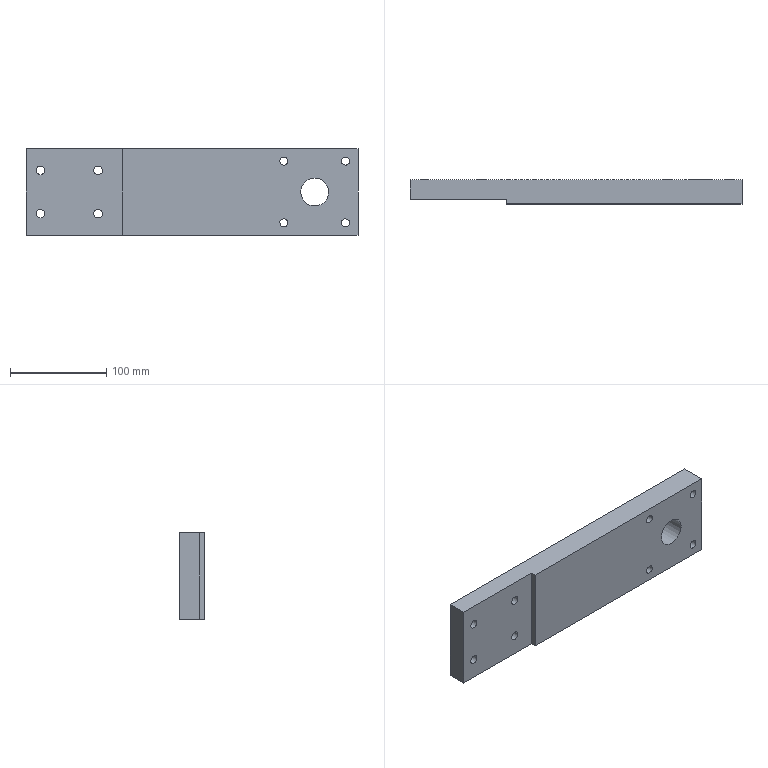Part | STEP file | SN10_001_007_PLACA | 1 solid | 17 faces | box 345 x 25 x 90 mm | volume 704137 mm3 | cylinder 9 | plane 8 | commonest cylinder face diameters 8.376 x4 9 x4 29 x1
STEP:
#1=CARTESIAN_POINT('',(0.,0.,0.));
#2=DIRECTION('',(0.,0.,1.));
#3=DIRECTION('',(1.,0.,0.));
#4=AXIS2_PLACEMENT_3D('',#1,#2,#3);
#5=CARTESIAN_POINT('',(5718.949,200.,-20.343));
#6=VERTEX_POINT('',#5);
#7=CARTESIAN_POINT('',(5715.,200.,-22.5));
#8=DIRECTION('',(0.,-1.,0.));
#9=DIRECTION('',(1.,0.,0.));
#10=AXIS2_PLACEMENT_3D('',#7,#8,#9);
#11=CIRCLE('',#10,4.5);
#12=CARTESIAN_POINT('',(5715.,199.9,-22.5));
#13=DIRECTION('',(0.,-1.,0.));
#14=DIRECTION('',(0.8776,0.,0.4794));
#15=AXIS2_PLACEMENT_3D('',#12,#13,#14);
#16=CYLINDRICAL_SURFACE('',#15,4.5);
#17=CARTESIAN_POINT('',(-0.5,-0.1));
#18=DIRECTION('',(1.,0.));
#19=VECTOR('',#18,1.);
#20=LINE('',#17,#19);
#21=(GEOMETRIC_REPRESENTATION_CONTEXT(2)PARAMETRIC_REPRESENTATION_CONTEXT()REPRESENTATION_CONTEXT('',''));
#22=DEFINITIONAL_REPRESENTATION('',(#20),#21);
#23=PCURVE('',#16,#22);
#24=CARTESIAN_POINT('',(6045.,200.,0.));
#25=DIRECTION('',(0.,1.,0.));
#26=DIRECTION('',(0.,0.,1.));
#27=AXIS2_PLACEMENT_3D('',#24,#25,#26);
#28=PLANE('',#27);
#29=CARTESIAN_POINT('',(-22.5,-325.5));
#30=CARTESIAN_POINT('',(-14.706,-325.5));
#31=CARTESIAN_POINT('',(-18.603,-332.25));
#32=CARTESIAN_POINT('',(-22.5,-339.));
#33=CARTESIAN_POINT('',(-26.397,-332.25));
#34=CARTESIAN_POINT('',(-30.294,-325.5));
#35=CARTESIAN_POINT('',(-22.5,-325.5));
#36=(BOUNDED_CURVE()B_SPLINE_CURVE(2,(#29,#30,#31,#32,#33,#34,#35),.UNSPECIFIED.,.T.,.F.)B_SPLINE_CURVE_WITH_KNOTS((1,2,2,2,2,1),(-2.094,0.,2.094,4.189,6.283,8.378),.UNSPECIFIED.)CURVE()GEOMETRIC_REPRESENTATION_ITEM()RATIONAL_B_SPLINE_CURVE((1.,0.5,1.,0.5,1.,0.5,1.))REPRESENTATION_ITEM(''));
#37=(GEOMETRIC_REPRESENTATION_CONTEXT(2)PARAMETRIC_REPRESENTATION_CONTEXT()REPRESENTATION_CONTEXT('',''));
#38=DEFINITIONAL_REPRESENTATION('',(#36),#37);
#39=PCURVE('',#28,#38);
#40=SURFACE_CURVE('',#11,(#23,#39),.PCURVE_S1.);
#41=EDGE_CURVE('',#6,#6,#40,.T.);
#42=ORIENTED_EDGE('',*,*,#41,.T.);
#43=CARTESIAN_POINT('',(5718.949,180.,-20.343));
#44=VERTEX_POINT('',#43);
#45=CARTESIAN_POINT('',(5718.949,200.,-20.343));
#46=CARTESIAN_POINT('',(5718.949,180.,-20.343));
#47=B_SPLINE_CURVE_WITH_KNOTS('',1,(#45,#46),.UNSPECIFIED.,.F.,.F.,(2,2),(-0.1,19.9),.PIECEWISE_BEZIER_KNOTS.);
#48=CARTESIAN_POINT('',(6.283,0.));
#49=DIRECTION('',(0.,1.));
#50=VECTOR('',#49,1.);
#51=LINE('',#48,#50);
#52=(GEOMETRIC_REPRESENTATION_CONTEXT(2)PARAMETRIC_REPRESENTATION_CONTEXT()REPRESENTATION_CONTEXT('',''));
#53=DEFINITIONAL_REPRESENTATION('',(#51),#52);
#54=PCURVE('',#16,#53);
#55=CARTESIAN_POINT('',(0.,0.));
#56=DIRECTION('',(0.,1.));
#57=VECTOR('',#56,1.);
#58=LINE('',#55,#57);
#59=(GEOMETRIC_REPRESENTATION_CONTEXT(2)PARAMETRIC_REPRESENTATION_CONTEXT()REPRESENTATION_CONTEXT('',''));
#60=DEFINITIONAL_REPRESENTATION('',(#58),#59);
#61=PCURVE('',#16,#60);
#62=SEAM_CURVE('',#47,(#54,#61),.PCURVE_S1.);
#63=EDGE_CURVE('',#6,#44,#62,.T.);
#64=ORIENTED_EDGE('',*,*,#63,.T.);
#65=CARTESIAN_POINT('',(5715.,180.,-22.5));
#66=DIRECTION('',(0.,-1.,0.));
#67=DIRECTION('',(1.,0.,0.));
#68=AXIS2_PLACEMENT_3D('',#65,#66,#67);
#69=CIRCLE('',#68,4.5);
#70=CARTESIAN_POINT('',(-0.5,19.9));
#71=DIRECTION('',(1.,0.));
#72=VECTOR('',#71,1.);
#73=LINE('',#70,#72);
#74=(GEOMETRIC_REPRESENTATION_CONTEXT(2)PARAMETRIC_REPRESENTATION_CONTEXT()REPRESENTATION_CONTEXT('',''));
#75=DEFINITIONAL_REPRESENTATION('',(#73),#74);
#76=PCURVE('',#16,#75);
#77=CARTESIAN_POINT('',(5700.,180.,0.));
#78=DIRECTION('',(0.,-1.,0.));
#79=DIRECTION('',(0.,0.,-1.));
#80=AXIS2_PLACEMENT_3D('',#77,#78,#79);
#81=PLANE('',#80);
#82=CARTESIAN_POINT('',(22.5,15.));
#83=DIRECTION('',(0.,1.));
#84=AXIS2_PLACEMENT_2D('',#82,#83);
#85=CIRCLE('',#84,4.5);
#86=(GEOMETRIC_REPRESENTATION_CONTEXT(2)PARAMETRIC_REPRESENTATION_CONTEXT()REPRESENTATION_CONTEXT('',''));
#87=DEFINITIONAL_REPRESENTATION('',(#85),#86);
#88=PCURVE('',#81,#87);
#89=SURFACE_CURVE('',#69,(#76,#88),.PCURVE_S1.);
#90=EDGE_CURVE('',#44,#44,#89,.T.);
#91=ORIENTED_EDGE('',*,*,#90,.F.);
#92=ORIENTED_EDGE('',*,*,#63,.F.);
#93=EDGE_LOOP('',(#42,#64,#91,#92));
#94=FACE_BOUND('',#93,.F.);
#95=ADVANCED_FACE('',(#94),#16,.F.);
#96=CARTESIAN_POINT('',(5700.,200.,-45.));
#97=VERTEX_POINT('',#96);
#98=CARTESIAN_POINT('',(5700.,180.,-45.));
#99=VERTEX_POINT('',#98);
#100=CARTESIAN_POINT('',(5700.,200.,-45.));
#101=DIRECTION('',(0.,-1.,0.));
#102=VECTOR('',#101,1.);
#103=LINE('',#100,#102);
#104=CARTESIAN_POINT('',(0.,0.,-45.));
#105=DIRECTION('',(0.,0.,1.));
#106=DIRECTION('',(1.,0.,0.));
#107=AXIS2_PLACEMENT_3D('',#104,#105,#106);
#108=PLANE('',#107);
#109=CARTESIAN_POINT('',(5700.,200.));
#110=DIRECTION('',(0.,-1.));
#111=VECTOR('',#110,1.);
#112=LINE('',#109,#111);
#113=(GEOMETRIC_REPRESENTATION_CONTEXT(2)PARAMETRIC_REPRESENTATION_CONTEXT()REPRESENTATION_CONTEXT('',''));
#114=DEFINITIONAL_REPRESENTATION('',(#112),#113);
#115=PCURVE('',#108,#114);
#116=CARTESIAN_POINT('',(5700.,200.,0.));
#117=DIRECTION('',(-1.,0.,0.));
#118=DIRECTION('',(0.,0.,1.));
#119=AXIS2_PLACEMENT_3D('',#116,#117,#118);
#120=PLANE('',#119);
#121=CARTESIAN_POINT('',(-45.,0.));
#122=DIRECTION('',(0.,-1.));
#123=VECTOR('',#122,1.);
#124=LINE('',#121,#123);
#125=(GEOMETRIC_REPRESENTATION_CONTEXT(2)PARAMETRIC_REPRESENTATION_CONTEXT()REPRESENTATION_CONTEXT('',''));
#126=DEFINITIONAL_REPRESENTATION('',(#124),#125);
#127=PCURVE('',#120,#126);
#128=SURFACE_CURVE('',#103,(#115,#127),.PCURVE_S1.);
#129=EDGE_CURVE('',#97,#99,#128,.T.);
#130=ORIENTED_EDGE('',*,*,#129,.F.);
#131=CARTESIAN_POINT('',(6045.,200.,-45.));
#132=VERTEX_POINT('',#131);
#133=CARTESIAN_POINT('',(6045.,200.,-45.));
#134=DIRECTION('',(-1.,0.,0.));
#135=VECTOR('',#134,1.);
#136=LINE('',#133,#135);
#137=CARTESIAN_POINT('',(6045.,200.));
#138=DIRECTION('',(-1.,0.));
#139=VECTOR('',#138,1.);
#140=LINE('',#137,#139);
#141=(GEOMETRIC_REPRESENTATION_CONTEXT(2)PARAMETRIC_REPRESENTATION_CONTEXT()REPRESENTATION_CONTEXT('',''));
#142=DEFINITIONAL_REPRESENTATION('',(#140),#141);
#143=PCURVE('',#108,#142);
#144=CARTESIAN_POINT('',(-45.,0.));
#145=DIRECTION('',(0.,-1.));
#146=VECTOR('',#145,1.);
#147=LINE('',#144,#146);
#148=(GEOMETRIC_REPRESENTATION_CONTEXT(2)PARAMETRIC_REPRESENTATION_CONTEXT()REPRESENTATION_CONTEXT('',''));
#149=DEFINITIONAL_REPRESENTATION('',(#147),#148);
#150=PCURVE('',#28,#149);
#151=SURFACE_CURVE('',#136,(#143,#150),.PCURVE_S1.);
#152=EDGE_CURVE('',#132,#97,#151,.T.);
#153=ORIENTED_EDGE('',*,*,#152,.F.);
#154=CARTESIAN_POINT('',(6045.,175.,-45.));
#155=VERTEX_POINT('',#154);
#156=CARTESIAN_POINT('',(6045.,175.,-45.));
#157=DIRECTION('',(0.,1.,0.));
#158=VECTOR('',#157,1.);
#159=LINE('',#156,#158);
#160=CARTESIAN_POINT('',(6045.,175.));
#161=DIRECTION('',(0.,1.));
#162=VECTOR('',#161,1.);
#163=LINE('',#160,#162);
#164=(GEOMETRIC_REPRESENTATION_CONTEXT(2)PARAMETRIC_REPRESENTATION_CONTEXT()REPRESENTATION_CONTEXT('',''));
#165=DEFINITIONAL_REPRESENTATION('',(#163),#164);
#166=PCURVE('',#108,#165);
#167=CARTESIAN_POINT('',(6045.,175.,0.));
#168=DIRECTION('',(1.,0.,0.));
#169=DIRECTION('',(0.,0.,-1.));
#170=AXIS2_PLACEMENT_3D('',#167,#168,#169);
#171=PLANE('',#170);
#172=CARTESIAN_POINT('',(45.,0.));
#173=DIRECTION('',(0.,1.));
#174=VECTOR('',#173,1.);
#175=LINE('',#172,#174);
#176=(GEOMETRIC_REPRESENTATION_CONTEXT(2)PARAMETRIC_REPRESENTATION_CONTEXT()REPRESENTATION_CONTEXT('',''));
#177=DEFINITIONAL_REPRESENTATION('',(#175),#176);
#178=PCURVE('',#171,#177);
#179=SURFACE_CURVE('',#159,(#166,#178),.PCURVE_S1.);
#180=EDGE_CURVE('',#155,#132,#179,.T.);
#181=ORIENTED_EDGE('',*,*,#180,.F.);
#182=CARTESIAN_POINT('',(5800.,175.,-45.));
#183=VERTEX_POINT('',#182);
#184=CARTESIAN_POINT('',(5800.,175.,-45.));
#185=DIRECTION('',(1.,0.,0.));
#186=VECTOR('',#185,1.);
#187=LINE('',#184,#186);
#188=CARTESIAN_POINT('',(5800.,175.));
#189=DIRECTION('',(1.,0.));
#190=VECTOR('',#189,1.);
#191=LINE('',#188,#190);
#192=(GEOMETRIC_REPRESENTATION_CONTEXT(2)PARAMETRIC_REPRESENTATION_CONTEXT()REPRESENTATION_CONTEXT('',''));
#193=DEFINITIONAL_REPRESENTATION('',(#191),#192);
#194=PCURVE('',#108,#193);
#195=CARTESIAN_POINT('',(5800.,175.,0.));
#196=DIRECTION('',(0.,-1.,0.));
#197=DIRECTION('',(0.,0.,-1.));
#198=AXIS2_PLACEMENT_3D('',#195,#196,#197);
#199=PLANE('',#198);
#200=CARTESIAN_POINT('',(45.,0.));
#201=DIRECTION('',(0.,1.));
#202=VECTOR('',#201,1.);
#203=LINE('',#200,#202);
#204=(GEOMETRIC_REPRESENTATION_CONTEXT(2)PARAMETRIC_REPRESENTATION_CONTEXT()REPRESENTATION_CONTEXT('',''));
#205=DEFINITIONAL_REPRESENTATION('',(#203),#204);
#206=PCURVE('',#199,#205);
#207=SURFACE_CURVE('',#187,(#194,#206),.PCURVE_S1.);
#208=EDGE_CURVE('',#183,#155,#207,.T.);
#209=ORIENTED_EDGE('',*,*,#208,.F.);
#210=CARTESIAN_POINT('',(5800.,180.,-45.));
#211=VERTEX_POINT('',#210);
#212=CARTESIAN_POINT('',(5800.,180.,-45.));
#213=DIRECTION('',(0.,-1.,0.));
#214=VECTOR('',#213,1.);
#215=LINE('',#212,#214);
#216=CARTESIAN_POINT('',(5800.,180.));
#217=DIRECTION('',(0.,-1.));
#218=VECTOR('',#217,1.);
#219=LINE('',#216,#218);
#220=(GEOMETRIC_REPRESENTATION_CONTEXT(2)PARAMETRIC_REPRESENTATION_CONTEXT()REPRESENTATION_CONTEXT('',''));
#221=DEFINITIONAL_REPRESENTATION('',(#219),#220);
#222=PCURVE('',#108,#221);
#223=CARTESIAN_POINT('',(5800.,180.,0.));
#224=DIRECTION('',(-1.,0.,0.));
#225=DIRECTION('',(0.,0.,1.));
#226=AXIS2_PLACEMENT_3D('',#223,#224,#225);
#227=PLANE('',#226);
#228=CARTESIAN_POINT('',(-45.,0.));
#229=DIRECTION('',(0.,-1.));
#230=VECTOR('',#229,1.);
#231=LINE('',#228,#230);
#232=(GEOMETRIC_REPRESENTATION_CONTEXT(2)PARAMETRIC_REPRESENTATION_CONTEXT()REPRESENTATION_CONTEXT('',''));
#233=DEFINITIONAL_REPRESENTATION('',(#231),#232);
#234=PCURVE('',#227,#233);
#235=SURFACE_CURVE('',#215,(#222,#234),.PCURVE_S1.);
#236=EDGE_CURVE('',#211,#183,#235,.T.);
#237=ORIENTED_EDGE('',*,*,#236,.F.);
#238=CARTESIAN_POINT('',(5700.,180.,-45.));
#239=DIRECTION('',(1.,0.,0.));
#240=VECTOR('',#239,1.);
#241=LINE('',#238,#240);
#242=CARTESIAN_POINT('',(5700.,180.));
#243=DIRECTION('',(1.,0.));
#244=VECTOR('',#243,1.);
#245=LINE('',#242,#244);
#246=(GEOMETRIC_REPRESENTATION_CONTEXT(2)PARAMETRIC_REPRESENTATION_CONTEXT()REPRESENTATION_CONTEXT('',''));
#247=DEFINITIONAL_REPRESENTATION('',(#245),#246);
#248=PCURVE('',#108,#247);
#249=CARTESIAN_POINT('',(45.,0.));
#250=DIRECTION('',(0.,1.));
#251=VECTOR('',#250,1.);
#252=LINE('',#249,#251);
#253=(GEOMETRIC_REPRESENTATION_CONTEXT(2)PARAMETRIC_REPRESENTATION_CONTEXT()REPRESENTATION_CONTEXT('',''));
#254=DEFINITIONAL_REPRESENTATION('',(#252),#253);
#255=PCURVE('',#81,#254);
#256=SURFACE_CURVE('',#241,(#248,#255),.PCURVE_S1.);
#257=EDGE_CURVE('',#99,#211,#256,.T.);
#258=ORIENTED_EDGE('',*,*,#257,.F.);
#259=EDGE_LOOP('',(#130,#153,#181,#209,#237,#258));
#260=FACE_BOUND('',#259,.T.);
#261=ADVANCED_FACE('',(#260),#108,.F.);
#262=CARTESIAN_POINT('',(5700.,200.,45.));
#263=VERTEX_POINT('',#262);
#264=CARTESIAN_POINT('',(5700.,200.,-45.));
#265=DIRECTION('',(0.,0.,1.));
#266=VECTOR('',#265,1.);
#267=LINE('',#264,#266);
#268=CARTESIAN_POINT('',(-45.,0.));
#269=DIRECTION('',(1.,0.));
#270=VECTOR('',#269,1.);
#271=LINE('',#268,#270);
#272=(GEOMETRIC_REPRESENTATION_CONTEXT(2)PARAMETRIC_REPRESENTATION_CONTEXT()REPRESENTATION_CONTEXT('',''));
#273=DEFINITIONAL_REPRESENTATION('',(#271),#272);
#274=PCURVE('',#120,#273);
#275=CARTESIAN_POINT('',(-45.,-345.));
#276=DIRECTION('',(1.,0.));
#277=VECTOR('',#276,1.);
#278=LINE('',#275,#277);
#279=(GEOMETRIC_REPRESENTATION_CONTEXT(2)PARAMETRIC_REPRESENTATION_CONTEXT()REPRESENTATION_CONTEXT('',''));
#280=DEFINITIONAL_REPRESENTATION('',(#278),#279);
#281=PCURVE('',#28,#280);
#282=SURFACE_CURVE('',#267,(#274,#281),.PCURVE_S1.);
#283=EDGE_CURVE('',#97,#263,#282,.T.);
#284=ORIENTED_EDGE('',*,*,#283,.F.);
#285=ORIENTED_EDGE('',*,*,#129,.T.);
#286=CARTESIAN_POINT('',(5700.,180.,45.));
#287=VERTEX_POINT('',#286);
#288=CARTESIAN_POINT('',(5700.,180.,-45.));
#289=DIRECTION('',(0.,0.,1.));
#290=VECTOR('',#289,1.);
#291=LINE('',#288,#290);
#292=CARTESIAN_POINT('',(-45.,-20.));
#293=DIRECTION('',(1.,0.));
#294=VECTOR('',#293,1.);
#295=LINE('',#292,#294);
#296=(GEOMETRIC_REPRESENTATION_CONTEXT(2)PARAMETRIC_REPRESENTATION_CONTEXT()REPRESENTATION_CONTEXT('',''));
#297=DEFINITIONAL_REPRESENTATION('',(#295),#296);
#298=PCURVE('',#120,#297);
#299=CARTESIAN_POINT('',(45.,0.));
#300=DIRECTION('',(-1.,0.));
#301=VECTOR('',#300,1.);
#302=LINE('',#299,#301);
#303=(GEOMETRIC_REPRESENTATION_CONTEXT(2)PARAMETRIC_REPRESENTATION_CONTEXT()REPRESENTATION_CONTEXT('',''));
#304=DEFINITIONAL_REPRESENTATION('',(#302),#303);
#305=PCURVE('',#81,#304);
#306=SURFACE_CURVE('',#291,(#298,#305),.PCURVE_S1.);
#307=EDGE_CURVE('',#99,#287,#306,.T.);
#308=ORIENTED_EDGE('',*,*,#307,.T.);
#309=CARTESIAN_POINT('',(5700.,200.,45.));
#310=DIRECTION('',(0.,-1.,0.));
#311=VECTOR('',#310,1.);
#312=LINE('',#309,#311);
#313=CARTESIAN_POINT('',(45.,0.));
#314=DIRECTION('',(0.,-1.));
#315=VECTOR('',#314,1.);
#316=LINE('',#313,#315);
#317=(GEOMETRIC_REPRESENTATION_CONTEXT(2)PARAMETRIC_REPRESENTATION_CONTEXT()REPRESENTATION_CONTEXT('',''));
#318=DEFINITIONAL_REPRESENTATION('',(#316),#317);
#319=PCURVE('',#120,#318);
#320=CARTESIAN_POINT('',(0.,0.,45.));
#321=DIRECTION('',(0.,0.,1.));
#322=DIRECTION('',(1.,0.,0.));
#323=AXIS2_PLACEMENT_3D('',#320,#321,#322);
#324=PLANE('',#323);
#325=CARTESIAN_POINT('',(5700.,200.));
#326=DIRECTION('',(0.,-1.));
#327=VECTOR('',#326,1.);
#328=LINE('',#325,#327);
#329=(GEOMETRIC_REPRESENTATION_CONTEXT(2)PARAMETRIC_REPRESENTATION_CONTEXT()REPRESENTATION_CONTEXT('',''));
#330=DEFINITIONAL_REPRESENTATION('',(#328),#329);
#331=PCURVE('',#324,#330);
#332=SURFACE_CURVE('',#312,(#319,#331),.PCURVE_S1.);
#333=EDGE_CURVE('',#263,#287,#332,.T.);
#334=ORIENTED_EDGE('',*,*,#333,.F.);
#335=EDGE_LOOP('',(#284,#285,#308,#334));
#336=FACE_BOUND('',#335,.T.);
#337=ADVANCED_FACE('',(#336),#120,.T.);
#338=CARTESIAN_POINT('',(5800.,180.,45.));
#339=VERTEX_POINT('',#338);
#340=CARTESIAN_POINT('',(5800.,180.,-45.));
#341=DIRECTION('',(0.,0.,1.));
#342=VECTOR('',#341,1.);
#343=LINE('',#340,#342);
#344=CARTESIAN_POINT('',(-45.,0.));
#345=DIRECTION('',(1.,0.));
#346=VECTOR('',#345,1.);
#347=LINE('',#344,#346);
#348=(GEOMETRIC_REPRESENTATION_CONTEXT(2)PARAMETRIC_REPRESENTATION_CONTEXT()REPRESENTATION_CONTEXT('',''));
#349=DEFINITIONAL_REPRESENTATION('',(#347),#348);
#350=PCURVE('',#227,#349);
#351=CARTESIAN_POINT('',(45.,100.));
#352=DIRECTION('',(-1.,0.));
#353=VECTOR('',#352,1.);
#354=LINE('',#351,#353);
#355=(GEOMETRIC_REPRESENTATION_CONTEXT(2)PARAMETRIC_REPRESENTATION_CONTEXT()REPRESENTATION_CONTEXT('',''));
#356=DEFINITIONAL_REPRESENTATION('',(#354),#355);
#357=PCURVE('',#81,#356);
#358=SURFACE_CURVE('',#343,(#350,#357),.PCURVE_S1.);
#359=EDGE_CURVE('',#211,#339,#358,.T.);
#360=ORIENTED_EDGE('',*,*,#359,.F.);
#361=ORIENTED_EDGE('',*,*,#236,.T.);
#362=CARTESIAN_POINT('',(5800.,175.,45.));
#363=VERTEX_POINT('',#362);
#364=CARTESIAN_POINT('',(5800.,175.,-45.));
#365=DIRECTION('',(0.,0.,1.));
#366=VECTOR('',#365,1.);
#367=LINE('',#364,#366);
#368=CARTESIAN_POINT('',(-45.,-5.));
#369=DIRECTION('',(1.,0.));
#370=VECTOR('',#369,1.);
#371=LINE('',#368,#370);
#372=(GEOMETRIC_REPRESENTATION_CONTEXT(2)PARAMETRIC_REPRESENTATION_CONTEXT()REPRESENTATION_CONTEXT('',''));
#373=DEFINITIONAL_REPRESENTATION('',(#371),#372);
#374=PCURVE('',#227,#373);
#375=CARTESIAN_POINT('',(45.,0.));
#376=DIRECTION('',(-1.,0.));
#377=VECTOR('',#376,1.);
#378=LINE('',#375,#377);
#379=(GEOMETRIC_REPRESENTATION_CONTEXT(2)PARAMETRIC_REPRESENTATION_CONTEXT()REPRESENTATION_CONTEXT('',''));
#380=DEFINITIONAL_REPRESENTATION('',(#378),#379);
#381=PCURVE('',#199,#380);
#382=SURFACE_CURVE('',#367,(#374,#381),.PCURVE_S1.);
#383=EDGE_CURVE('',#183,#363,#382,.T.);
#384=ORIENTED_EDGE('',*,*,#383,.T.);
#385=CARTESIAN_POINT('',(5800.,180.,45.));
#386=DIRECTION('',(0.,-1.,0.));
#387=VECTOR('',#386,1.);
#388=LINE('',#385,#387);
#389=CARTESIAN_POINT('',(45.,0.));
#390=DIRECTION('',(0.,-1.));
#391=VECTOR('',#390,1.);
#392=LINE('',#389,#391);
#393=(GEOMETRIC_REPRESENTATION_CONTEXT(2)PARAMETRIC_REPRESENTATION_CONTEXT()REPRESENTATION_CONTEXT('',''));
#394=DEFINITIONAL_REPRESENTATION('',(#392),#393);
#395=PCURVE('',#227,#394);
#396=CARTESIAN_POINT('',(5800.,180.));
#397=DIRECTION('',(0.,-1.));
#398=VECTOR('',#397,1.);
#399=LINE('',#396,#398);
#400=(GEOMETRIC_REPRESENTATION_CONTEXT(2)PARAMETRIC_REPRESENTATION_CONTEXT()REPRESENTATION_CONTEXT('',''));
#401=DEFINITIONAL_REPRESENTATION('',(#399),#400);
#402=PCURVE('',#324,#401);
#403=SURFACE_CURVE('',#388,(#395,#402),.PCURVE_S1.);
#404=EDGE_CURVE('',#339,#363,#403,.T.);
#405=ORIENTED_EDGE('',*,*,#404,.F.);
#406=EDGE_LOOP('',(#360,#361,#384,#405));
#407=FACE_BOUND('',#406,.T.);
#408=ADVANCED_FACE('',(#407),#227,.T.);
#409=ORIENTED_EDGE('',*,*,#383,.F.);
#410=ORIENTED_EDGE('',*,*,#208,.T.);
#411=CARTESIAN_POINT('',(6045.,175.,45.));
#412=VERTEX_POINT('',#411);
#413=CARTESIAN_POINT('',(6045.,175.,-45.));
#414=DIRECTION('',(0.,0.,1.));
#415=VECTOR('',#414,1.);
#416=LINE('',#413,#415);
#417=CARTESIAN_POINT('',(45.,245.));
#418=DIRECTION('',(-1.,0.));
#419=VECTOR('',#418,1.);
#420=LINE('',#417,#419);
#421=(GEOMETRIC_REPRESENTATION_CONTEXT(2)PARAMETRIC_REPRESENTATION_CONTEXT()REPRESENTATION_CONTEXT('',''));
#422=DEFINITIONAL_REPRESENTATION('',(#420),#421);
#423=PCURVE('',#199,#422);
#424=CARTESIAN_POINT('',(45.,0.));
#425=DIRECTION('',(-1.,0.));
#426=VECTOR('',#425,1.);
#427=LINE('',#424,#426);
#428=(GEOMETRIC_REPRESENTATION_CONTEXT(2)PARAMETRIC_REPRESENTATION_CONTEXT()REPRESENTATION_CONTEXT('',''));
#429=DEFINITIONAL_REPRESENTATION('',(#427),#428);
#430=PCURVE('',#171,#429);
#431=SURFACE_CURVE('',#416,(#423,#430),.PCURVE_S1.);
#432=EDGE_CURVE('',#155,#412,#431,.T.);
#433=ORIENTED_EDGE('',*,*,#432,.T.);
#434=CARTESIAN_POINT('',(5800.,175.,45.));
#435=DIRECTION('',(1.,0.,0.));
#436=VECTOR('',#435,1.);
#437=LINE('',#434,#436);
#438=CARTESIAN_POINT('',(-45.,0.));
#439=DIRECTION('',(0.,1.));
#440=VECTOR('',#439,1.);
#441=LINE('',#438,#440);
#442=(GEOMETRIC_REPRESENTATION_CONTEXT(2)PARAMETRIC_REPRESENTATION_CONTEXT()REPRESENTATION_CONTEXT('',''));
#443=DEFINITIONAL_REPRESENTATION('',(#441),#442);
#444=PCURVE('',#199,#443);
#445=CARTESIAN_POINT('',(5800.,175.));
#446=DIRECTION('',(1.,0.));
#447=VECTOR('',#446,1.);
#448=LINE('',#445,#447);
#449=(GEOMETRIC_REPRESENTATION_CONTEXT(2)PARAMETRIC_REPRESENTATION_CONTEXT()REPRESENTATION_CONTEXT('',''));
#450=DEFINITIONAL_REPRESENTATION('',(#448),#449);
#451=PCURVE('',#324,#450);
#452=SURFACE_CURVE('',#437,(#444,#451),.PCURVE_S1.);
#453=EDGE_CURVE('',#363,#412,#452,.T.);
#454=ORIENTED_EDGE('',*,*,#453,.F.);
#455=EDGE_LOOP('',(#409,#410,#433,#454));
#456=FACE_BOUND('',#455,.T.);
#457=CARTESIAN_POINT('',(6035.675,175.,34.008));
#458=VERTEX_POINT('',#457);
#459=CARTESIAN_POINT('',(6032.,175.,32.));
#460=DIRECTION('',(0.,-1.,0.));
#461=DIRECTION('',(1.,0.,0.));
#462=AXIS2_PLACEMENT_3D('',#459,#460,#461);
#463=CIRCLE('',#462,4.188);
#464=CARTESIAN_POINT('',(-32.,232.));
#465=DIRECTION('',(0.,1.));
#466=AXIS2_PLACEMENT_2D('',#464,#465);
#467=CIRCLE('',#466,4.188);
#468=(GEOMETRIC_REPRESENTATION_CONTEXT(2)PARAMETRIC_REPRESENTATION_CONTEXT()REPRESENTATION_CONTEXT('',''));
#469=DEFINITIONAL_REPRESENTATION('',(#467),#468);
#470=PCURVE('',#199,#469);
#471=CARTESIAN_POINT('',(6032.,199.9,32.));
#472=DIRECTION('',(0.,-1.,0.));
#473=DIRECTION('',(0.8776,0.,0.4794));
#474=AXIS2_PLACEMENT_3D('',#471,#472,#473);
#475=CYLINDRICAL_SURFACE('',#474,4.188);
#476=CARTESIAN_POINT('',(-0.5,24.9));
#477=DIRECTION('',(1.,0.));
#478=VECTOR('',#477,1.);
#479=LINE('',#476,#478);
#480=(GEOMETRIC_REPRESENTATION_CONTEXT(2)PARAMETRIC_REPRESENTATION_CONTEXT()REPRESENTATION_CONTEXT('',''));
#481=DEFINITIONAL_REPRESENTATION('',(#479),#480);
#482=PCURVE('',#475,#481);
#483=SURFACE_CURVE('',#463,(#470,#482),.PCURVE_S1.);
#484=EDGE_CURVE('',#458,#458,#483,.T.);
#485=ORIENTED_EDGE('',*,*,#484,.F.);
#486=EDGE_LOOP('',(#485));
#487=FACE_BOUND('',#486,.T.);
#488=CARTESIAN_POINT('',(5971.675,175.,34.008));
#489=VERTEX_POINT('',#488);
#490=CARTESIAN_POINT('',(5968.,175.,32.));
#491=DIRECTION('',(0.,-1.,0.));
#492=DIRECTION('',(1.,0.,0.));
#493=AXIS2_PLACEMENT_3D('',#490,#491,#492);
#494=CIRCLE('',#493,4.188);
#495=CARTESIAN_POINT('',(-32.,168.));
#496=DIRECTION('',(0.,1.));
#497=AXIS2_PLACEMENT_2D('',#495,#496);
#498=CIRCLE('',#497,4.188);
#499=(GEOMETRIC_REPRESENTATION_CONTEXT(2)PARAMETRIC_REPRESENTATION_CONTEXT()REPRESENTATION_CONTEXT('',''));
#500=DEFINITIONAL_REPRESENTATION('',(#498),#499);
#501=PCURVE('',#199,#500);
#502=CARTESIAN_POINT('',(5968.,199.9,32.));
#503=DIRECTION('',(0.,-1.,0.));
#504=DIRECTION('',(0.8776,0.,0.4794));
#505=AXIS2_PLACEMENT_3D('',#502,#503,#504);
#506=CYLINDRICAL_SURFACE('',#505,4.188);
#507=CARTESIAN_POINT('',(-0.5,24.9));
#508=DIRECTION('',(1.,0.));
#509=VECTOR('',#508,1.);
#510=LINE('',#507,#509);
#511=(GEOMETRIC_REPRESENTATION_CONTEXT(2)PARAMETRIC_REPRESENTATION_CONTEXT()REPRESENTATION_CONTEXT('',''));
#512=DEFINITIONAL_REPRESENTATION('',(#510),#511);
#513=PCURVE('',#506,#512);
#514=SURFACE_CURVE('',#494,(#501,#513),.PCURVE_S1.);
#515=EDGE_CURVE('',#489,#489,#514,.T.);
#516=ORIENTED_EDGE('',*,*,#515,.F.);
#517=EDGE_LOOP('',(#516));
#518=FACE_BOUND('',#517,.T.);
#519=CARTESIAN_POINT('',(5971.675,175.,-29.992));
#520=VERTEX_POINT('',#519);
#521=CARTESIAN_POINT('',(5968.,175.,-32.));
#522=DIRECTION('',(0.,-1.,0.));
#523=DIRECTION('',(1.,0.,0.));
#524=AXIS2_PLACEMENT_3D('',#521,#522,#523);
#525=CIRCLE('',#524,4.188);
#526=CARTESIAN_POINT('',(32.,168.));
#527=DIRECTION('',(0.,1.));
#528=AXIS2_PLACEMENT_2D('',#526,#527);
#529=CIRCLE('',#528,4.188);
#530=(GEOMETRIC_REPRESENTATION_CONTEXT(2)PARAMETRIC_REPRESENTATION_CONTEXT()REPRESENTATION_CONTEXT('',''));
#531=DEFINITIONAL_REPRESENTATION('',(#529),#530);
#532=PCURVE('',#199,#531);
#533=CARTESIAN_POINT('',(5968.,199.9,-32.));
#534=DIRECTION('',(0.,-1.,0.));
#535=DIRECTION('',(0.8776,0.,0.4794));
#536=AXIS2_PLACEMENT_3D('',#533,#534,#535);
#537=CYLINDRICAL_SURFACE('',#536,4.188);
#538=CARTESIAN_POINT('',(-0.5,24.9));
#539=DIRECTION('',(1.,0.));
#540=VECTOR('',#539,1.);
#541=LINE('',#538,#540);
#542=(GEOMETRIC_REPRESENTATION_CONTEXT(2)PARAMETRIC_REPRESENTATION_CONTEXT()REPRESENTATION_CONTEXT('',''));
#543=DEFINITIONAL_REPRESENTATION('',(#541),#542);
#544=PCURVE('',#537,#543);
#545=SURFACE_CURVE('',#525,(#532,#544),.PCURVE_S1.);
#546=EDGE_CURVE('',#520,#520,#545,.T.);
#547=ORIENTED_EDGE('',*,*,#546,.F.);
#548=EDGE_LOOP('',(#547));
#549=FACE_BOUND('',#548,.T.);
#550=CARTESIAN_POINT('',(6035.675,175.,-29.992));
#551=VERTEX_POINT('',#550);
#552=CARTESIAN_POINT('',(6032.,175.,-32.));
#553=DIRECTION('',(0.,-1.,0.));
#554=DIRECTION('',(1.,0.,0.));
#555=AXIS2_PLACEMENT_3D('',#552,#553,#554);
#556=CIRCLE('',#555,4.188);
#557=CARTESIAN_POINT('',(32.,232.));
#558=DIRECTION('',(0.,1.));
#559=AXIS2_PLACEMENT_2D('',#557,#558);
#560=CIRCLE('',#559,4.188);
#561=(GEOMETRIC_REPRESENTATION_CONTEXT(2)PARAMETRIC_REPRESENTATION_CONTEXT()REPRESENTATION_CONTEXT('',''));
#562=DEFINITIONAL_REPRESENTATION('',(#560),#561);
#563=PCURVE('',#199,#562);
#564=CARTESIAN_POINT('',(6032.,199.9,-32.));
#565=DIRECTION('',(0.,-1.,0.));
#566=DIRECTION('',(0.8776,0.,0.4794));
#567=AXIS2_PLACEMENT_3D('',#564,#565,#566);
#568=CYLINDRICAL_SURFACE('',#567,4.188);
#569=CARTESIAN_POINT('',(-0.5,24.9));
#570=DIRECTION('',(1.,0.));
#571=VECTOR('',#570,1.);
#572=LINE('',#569,#571);
#573=(GEOMETRIC_REPRESENTATION_CONTEXT(2)PARAMETRIC_REPRESENTATION_CONTEXT()REPRESENTATION_CONTEXT('',''));
#574=DEFINITIONAL_REPRESENTATION('',(#572),#573);
#575=PCURVE('',#568,#574);
#576=SURFACE_CURVE('',#556,(#563,#575),.PCURVE_S1.);
#577=EDGE_CURVE('',#551,#551,#576,.T.);
#578=ORIENTED_EDGE('',*,*,#577,.F.);
#579=EDGE_LOOP('',(#578));
#580=FACE_BOUND('',#579,.T.);
#581=CARTESIAN_POINT('',(6012.725,175.,6.952));
#582=VERTEX_POINT('',#581);
#583=CARTESIAN_POINT('',(6000.,175.,0.));
#584=DIRECTION('',(0.,-1.,0.));
#585=DIRECTION('',(1.,0.,0.));
#586=AXIS2_PLACEMENT_3D('',#583,#584,#585);
#587=CIRCLE('',#586,14.5);
#588=CARTESIAN_POINT('',(0.,200.));
#589=DIRECTION('',(0.,1.));
#590=AXIS2_PLACEMENT_2D('',#588,#589);
#591=CIRCLE('',#590,14.5);
#592=(GEOMETRIC_REPRESENTATION_CONTEXT(2)PARAMETRIC_REPRESENTATION_CONTEXT()REPRESENTATION_CONTEXT('',''));
#593=DEFINITIONAL_REPRESENTATION('',(#591),#592);
#594=PCURVE('',#199,#593);
#595=CARTESIAN_POINT('',(6000.,199.9,0.));
#596=DIRECTION('',(0.,-1.,0.));
#597=DIRECTION('',(0.8776,0.,0.4794));
#598=AXIS2_PLACEMENT_3D('',#595,#596,#597);
#599=CYLINDRICAL_SURFACE('',#598,14.5);
#600=CARTESIAN_POINT('',(-0.5,24.9));
#601=DIRECTION('',(1.,0.));
#602=VECTOR('',#601,1.);
#603=LINE('',#600,#602);
#604=(GEOMETRIC_REPRESENTATION_CONTEXT(2)PARAMETRIC_REPRESENTATION_CONTEXT()REPRESENTATION_CONTEXT('',''));
#605=DEFINITIONAL_REPRESENTATION('',(#603),#604);
#606=PCURVE('',#599,#605);
#607=SURFACE_CURVE('',#587,(#594,#606),.PCURVE_S1.);
#608=EDGE_CURVE('',#582,#582,#607,.T.);
#609=ORIENTED_EDGE('',*,*,#608,.F.);
#610=EDGE_LOOP('',(#609));
#611=FACE_BOUND('',#610,.T.);
#612=ADVANCED_FACE('',(#456,#487,#518,#549,#580,#611),#199,.T.);
#613=CARTESIAN_POINT('',(6012.725,200.,6.952));
#614=VERTEX_POINT('',#613);
#615=CARTESIAN_POINT('',(6000.,200.,0.));
#616=DIRECTION('',(0.,-1.,0.));
#617=DIRECTION('',(1.,0.,0.));
#618=AXIS2_PLACEMENT_3D('',#615,#616,#617);
#619=CIRCLE('',#618,14.5);
#620=CARTESIAN_POINT('',(-0.5,-0.1));
#621=DIRECTION('',(1.,0.));
#622=VECTOR('',#621,1.);
#623=LINE('',#620,#622);
#624=(GEOMETRIC_REPRESENTATION_CONTEXT(2)PARAMETRIC_REPRESENTATION_CONTEXT()REPRESENTATION_CONTEXT('',''));
#625=DEFINITIONAL_REPRESENTATION('',(#623),#624);
#626=PCURVE('',#599,#625);
#627=CARTESIAN_POINT('',(0.,-30.5));
#628=CARTESIAN_POINT('',(25.115,-30.5));
#629=CARTESIAN_POINT('',(12.557,-52.25));
#630=CARTESIAN_POINT('',(0.,-74.));
#631=CARTESIAN_POINT('',(-12.557,-52.25));
#632=CARTESIAN_POINT('',(-25.115,-30.5));
#633=CARTESIAN_POINT('',(0.,-30.5));
#634=(BOUNDED_CURVE()B_SPLINE_CURVE(2,(#627,#628,#629,#630,#631,#632,#633),.UNSPECIFIED.,.T.,.F.)B_SPLINE_CURVE_WITH_KNOTS((1,2,2,2,2,1),(-2.094,0.,2.094,4.189,6.283,8.378),.UNSPECIFIED.)CURVE()GEOMETRIC_REPRESENTATION_ITEM()RATIONAL_B_SPLINE_CURVE((1.,0.5,1.,0.5,1.,0.5,1.))REPRESENTATION_ITEM(''));
#635=(GEOMETRIC_REPRESENTATION_CONTEXT(2)PARAMETRIC_REPRESENTATION_CONTEXT()REPRESENTATION_CONTEXT('',''));
#636=DEFINITIONAL_REPRESENTATION('',(#634),#635);
#637=PCURVE('',#28,#636);
#638=SURFACE_CURVE('',#619,(#626,#637),.PCURVE_S1.);
#639=EDGE_CURVE('',#614,#614,#638,.T.);
#640=ORIENTED_EDGE('',*,*,#639,.T.);
#641=CARTESIAN_POINT('',(6012.725,200.,6.952));
#642=CARTESIAN_POINT('',(6012.725,175.,6.952));
#643=B_SPLINE_CURVE_WITH_KNOTS('',1,(#641,#642),.UNSPECIFIED.,.F.,.F.,(2,2),(-0.1,24.9),.PIECEWISE_BEZIER_KNOTS.);
#644=CARTESIAN_POINT('',(6.283,0.));
#645=DIRECTION('',(0.,1.));
#646=VECTOR('',#645,1.);
#647=LINE('',#644,#646);
#648=(GEOMETRIC_REPRESENTATION_CONTEXT(2)PARAMETRIC_REPRESENTATION_CONTEXT()REPRESENTATION_CONTEXT('',''));
#649=DEFINITIONAL_REPRESENTATION('',(#647),#648);
#650=PCURVE('',#599,#649);
#651=CARTESIAN_POINT('',(0.,0.));
#652=DIRECTION('',(0.,1.));
#653=VECTOR('',#652,1.);
#654=LINE('',#651,#653);
#655=(GEOMETRIC_REPRESENTATION_CONTEXT(2)PARAMETRIC_REPRESENTATION_CONTEXT()REPRESENTATION_CONTEXT('',''));
#656=DEFINITIONAL_REPRESENTATION('',(#654),#655);
#657=PCURVE('',#599,#656);
#658=SEAM_CURVE('',#643,(#650,#657),.PCURVE_S1.);
#659=EDGE_CURVE('',#614,#582,#658,.T.);
#660=ORIENTED_EDGE('',*,*,#659,.T.);
#661=ORIENTED_EDGE('',*,*,#608,.F.);
#662=ORIENTED_EDGE('',*,*,#659,.F.);
#663=EDGE_LOOP('',(#640,#660,#661,#662));
#664=FACE_BOUND('',#663,.F.);
#665=ADVANCED_FACE('',(#664),#599,.F.);
#666=CARTESIAN_POINT('',(6035.675,200.,-29.992));
#667=VERTEX_POINT('',#666);
#668=CARTESIAN_POINT('',(6032.,200.,-32.));
#669=DIRECTION('',(0.,-1.,0.));
#670=DIRECTION('',(1.,0.,0.));
#671=AXIS2_PLACEMENT_3D('',#668,#669,#670);
#672=CIRCLE('',#671,4.188);
#673=CARTESIAN_POINT('',(-0.5,-0.1));
#674=DIRECTION('',(1.,0.));
#675=VECTOR('',#674,1.);
#676=LINE('',#673,#675);
#677=(GEOMETRIC_REPRESENTATION_CONTEXT(2)PARAMETRIC_REPRESENTATION_CONTEXT()REPRESENTATION_CONTEXT('',''));
#678=DEFINITIONAL_REPRESENTATION('',(#676),#677);
#679=PCURVE('',#568,#678);
#680=CARTESIAN_POINT('',(-32.,-8.812));
#681=CARTESIAN_POINT('',(-24.746,-8.812));
#682=CARTESIAN_POINT('',(-28.373,-15.094));
#683=CARTESIAN_POINT('',(-32.,-21.376));
#684=CARTESIAN_POINT('',(-35.627,-15.094));
#685=CARTESIAN_POINT('',(-39.254,-8.812));
#686=CARTESIAN_POINT('',(-32.,-8.812));
#687=(BOUNDED_CURVE()B_SPLINE_CURVE(2,(#680,#681,#682,#683,#684,#685,#686),.UNSPECIFIED.,.T.,.F.)B_SPLINE_CURVE_WITH_KNOTS((1,2,2,2,2,1),(-2.094,0.,2.094,4.189,6.283,8.378),.UNSPECIFIED.)CURVE()GEOMETRIC_REPRESENTATION_ITEM()RATIONAL_B_SPLINE_CURVE((1.,0.5,1.,0.5,1.,0.5,1.))REPRESENTATION_ITEM(''));
#688=(GEOMETRIC_REPRESENTATION_CONTEXT(2)PARAMETRIC_REPRESENTATION_CONTEXT()REPRESENTATION_CONTEXT('',''));
#689=DEFINITIONAL_REPRESENTATION('',(#687),#688);
#690=PCURVE('',#28,#689);
#691=SURFACE_CURVE('',#672,(#679,#690),.PCURVE_S1.);
#692=EDGE_CURVE('',#667,#667,#691,.T.);
#693=ORIENTED_EDGE('',*,*,#692,.T.);
#694=CARTESIAN_POINT('',(6035.675,200.,-29.992));
#695=CARTESIAN_POINT('',(6035.675,175.,-29.992));
#696=B_SPLINE_CURVE_WITH_KNOTS('',1,(#694,#695),.UNSPECIFIED.,.F.,.F.,(2,2),(-0.1,24.9),.PIECEWISE_BEZIER_KNOTS.);
#697=CARTESIAN_POINT('',(6.283,0.));
#698=DIRECTION('',(0.,1.));
#699=VECTOR('',#698,1.);
#700=LINE('',#697,#699);
#701=(GEOMETRIC_REPRESENTATION_CONTEXT(2)PARAMETRIC_REPRESENTATION_CONTEXT()REPRESENTATION_CONTEXT('',''));
#702=DEFINITIONAL_REPRESENTATION('',(#700),#701);
#703=PCURVE('',#568,#702);
#704=CARTESIAN_POINT('',(0.,0.));
#705=DIRECTION('',(0.,1.));
#706=VECTOR('',#705,1.);
#707=LINE('',#704,#706);
#708=(GEOMETRIC_REPRESENTATION_CONTEXT(2)PARAMETRIC_REPRESENTATION_CONTEXT()REPRESENTATION_CONTEXT('',''));
#709=DEFINITIONAL_REPRESENTATION('',(#707),#708);
#710=PCURVE('',#568,#709);
#711=SEAM_CURVE('',#696,(#703,#710),.PCURVE_S1.);
#712=EDGE_CURVE('',#667,#551,#711,.T.);
#713=ORIENTED_EDGE('',*,*,#712,.T.);
#714=ORIENTED_EDGE('',*,*,#577,.F.);
#715=ORIENTED_EDGE('',*,*,#712,.F.);
#716=EDGE_LOOP('',(#693,#713,#714,#715));
#717=FACE_BOUND('',#716,.F.);
#718=ADVANCED_FACE('',(#717),#568,.F.);
#719=CARTESIAN_POINT('',(5971.675,200.,-29.992));
#720=VERTEX_POINT('',#719);
#721=CARTESIAN_POINT('',(5968.,200.,-32.));
#722=DIRECTION('',(0.,-1.,0.));
#723=DIRECTION('',(1.,0.,0.));
#724=AXIS2_PLACEMENT_3D('',#721,#722,#723);
#725=CIRCLE('',#724,4.188);
#726=CARTESIAN_POINT('',(-0.5,-0.1));
#727=DIRECTION('',(1.,0.));
#728=VECTOR('',#727,1.);
#729=LINE('',#726,#728);
#730=(GEOMETRIC_REPRESENTATION_CONTEXT(2)PARAMETRIC_REPRESENTATION_CONTEXT()REPRESENTATION_CONTEXT('',''));
#731=DEFINITIONAL_REPRESENTATION('',(#729),#730);
#732=PCURVE('',#537,#731);
#733=CARTESIAN_POINT('',(-32.,-72.812));
#734=CARTESIAN_POINT('',(-24.746,-72.812));
#735=CARTESIAN_POINT('',(-28.373,-79.094));
#736=CARTESIAN_POINT('',(-32.,-85.376));
#737=CARTESIAN_POINT('',(-35.627,-79.094));
#738=CARTESIAN_POINT('',(-39.254,-72.812));
#739=CARTESIAN_POINT('',(-32.,-72.812));
#740=(BOUNDED_CURVE()B_SPLINE_CURVE(2,(#733,#734,#735,#736,#737,#738,#739),.UNSPECIFIED.,.T.,.F.)B_SPLINE_CURVE_WITH_KNOTS((1,2,2,2,2,1),(-2.094,0.,2.094,4.189,6.283,8.378),.UNSPECIFIED.)CURVE()GEOMETRIC_REPRESENTATION_ITEM()RATIONAL_B_SPLINE_CURVE((1.,0.5,1.,0.5,1.,0.5,1.))REPRESENTATION_ITEM(''));
#741=(GEOMETRIC_REPRESENTATION_CONTEXT(2)PARAMETRIC_REPRESENTATION_CONTEXT()REPRESENTATION_CONTEXT('',''));
#742=DEFINITIONAL_REPRESENTATION('',(#740),#741);
#743=PCURVE('',#28,#742);
#744=SURFACE_CURVE('',#725,(#732,#743),.PCURVE_S1.);
#745=EDGE_CURVE('',#720,#720,#744,.T.);
#746=ORIENTED_EDGE('',*,*,#745,.T.);
#747=CARTESIAN_POINT('',(5971.675,200.,-29.992));
#748=CARTESIAN_POINT('',(5971.675,175.,-29.992));
#749=B_SPLINE_CURVE_WITH_KNOTS('',1,(#747,#748),.UNSPECIFIED.,.F.,.F.,(2,2),(-0.1,24.9),.PIECEWISE_BEZIER_KNOTS.);
#750=CARTESIAN_POINT('',(6.283,0.));
#751=DIRECTION('',(0.,1.));
#752=VECTOR('',#751,1.);
#753=LINE('',#750,#752);
#754=(GEOMETRIC_REPRESENTATION_CONTEXT(2)PARAMETRIC_REPRESENTATION_CONTEXT()REPRESENTATION_CONTEXT('',''));
#755=DEFINITIONAL_REPRESENTATION('',(#753),#754);
#756=PCURVE('',#537,#755);
#757=CARTESIAN_POINT('',(0.,0.));
#758=DIRECTION('',(0.,1.));
#759=VECTOR('',#758,1.);
#760=LINE('',#757,#759);
#761=(GEOMETRIC_REPRESENTATION_CONTEXT(2)PARAMETRIC_REPRESENTATION_CONTEXT()REPRESENTATION_CONTEXT('',''));
#762=DEFINITIONAL_REPRESENTATION('',(#760),#761);
#763=PCURVE('',#537,#762);
#764=SEAM_CURVE('',#749,(#756,#763),.PCURVE_S1.);
#765=EDGE_CURVE('',#720,#520,#764,.T.);
#766=ORIENTED_EDGE('',*,*,#765,.T.);
#767=ORIENTED_EDGE('',*,*,#546,.F.);
#768=ORIENTED_EDGE('',*,*,#765,.F.);
#769=EDGE_LOOP('',(#746,#766,#767,#768));
#770=FACE_BOUND('',#769,.F.);
#771=ADVANCED_FACE('',(#770),#537,.F.);
#772=CARTESIAN_POINT('',(5971.675,200.,34.008));
#773=VERTEX_POINT('',#772);
#774=CARTESIAN_POINT('',(5968.,200.,32.));
#775=DIRECTION('',(0.,-1.,0.));
#776=DIRECTION('',(1.,0.,0.));
#777=AXIS2_PLACEMENT_3D('',#774,#775,#776);
#778=CIRCLE('',#777,4.188);
#779=CARTESIAN_POINT('',(-0.5,-0.1));
#780=DIRECTION('',(1.,0.));
#781=VECTOR('',#780,1.);
#782=LINE('',#779,#781);
#783=(GEOMETRIC_REPRESENTATION_CONTEXT(2)PARAMETRIC_REPRESENTATION_CONTEXT()REPRESENTATION_CONTEXT('',''));
#784=DEFINITIONAL_REPRESENTATION('',(#782),#783);
#785=PCURVE('',#506,#784);
#786=CARTESIAN_POINT('',(32.,-72.812));
#787=CARTESIAN_POINT('',(39.254,-72.812));
#788=CARTESIAN_POINT('',(35.627,-79.094));
#789=CARTESIAN_POINT('',(32.,-85.376));
#790=CARTESIAN_POINT('',(28.373,-79.094));
#791=CARTESIAN_POINT('',(24.746,-72.812));
#792=CARTESIAN_POINT('',(32.,-72.812));
#793=(BOUNDED_CURVE()B_SPLINE_CURVE(2,(#786,#787,#788,#789,#790,#791,#792),.UNSPECIFIED.,.T.,.F.)B_SPLINE_CURVE_WITH_KNOTS((1,2,2,2,2,1),(-2.094,0.,2.094,4.189,6.283,8.378),.UNSPECIFIED.)CURVE()GEOMETRIC_REPRESENTATION_ITEM()RATIONAL_B_SPLINE_CURVE((1.,0.5,1.,0.5,1.,0.5,1.))REPRESENTATION_ITEM(''));
#794=(GEOMETRIC_REPRESENTATION_CONTEXT(2)PARAMETRIC_REPRESENTATION_CONTEXT()REPRESENTATION_CONTEXT('',''));
#795=DEFINITIONAL_REPRESENTATION('',(#793),#794);
#796=PCURVE('',#28,#795);
#797=SURFACE_CURVE('',#778,(#785,#796),.PCURVE_S1.);
#798=EDGE_CURVE('',#773,#773,#797,.T.);
#799=ORIENTED_EDGE('',*,*,#798,.T.);
#800=CARTESIAN_POINT('',(5971.675,200.,34.008));
#801=CARTESIAN_POINT('',(5971.675,175.,34.008));
#802=B_SPLINE_CURVE_WITH_KNOTS('',1,(#800,#801),.UNSPECIFIED.,.F.,.F.,(2,2),(-0.1,24.9),.PIECEWISE_BEZIER_KNOTS.);
#803=CARTESIAN_POINT('',(6.283,0.));
#804=DIRECTION('',(0.,1.));
#805=VECTOR('',#804,1.);
#806=LINE('',#803,#805);
#807=(GEOMETRIC_REPRESENTATION_CONTEXT(2)PARAMETRIC_REPRESENTATION_CONTEXT()REPRESENTATION_CONTEXT('',''));
#808=DEFINITIONAL_REPRESENTATION('',(#806),#807);
#809=PCURVE('',#506,#808);
#810=CARTESIAN_POINT('',(0.,0.));
#811=DIRECTION('',(0.,1.));
#812=VECTOR('',#811,1.);
#813=LINE('',#810,#812);
#814=(GEOMETRIC_REPRESENTATION_CONTEXT(2)PARAMETRIC_REPRESENTATION_CONTEXT()REPRESENTATION_CONTEXT('',''));
#815=DEFINITIONAL_REPRESENTATION('',(#813),#814);
#816=PCURVE('',#506,#815);
#817=SEAM_CURVE('',#802,(#809,#816),.PCURVE_S1.);
#818=EDGE_CURVE('',#773,#489,#817,.T.);
#819=ORIENTED_EDGE('',*,*,#818,.T.);
#820=ORIENTED_EDGE('',*,*,#515,.F.);
#821=ORIENTED_EDGE('',*,*,#818,.F.);
#822=EDGE_LOOP('',(#799,#819,#820,#821));
#823=FACE_BOUND('',#822,.F.);
#824=ADVANCED_FACE('',(#823),#506,.F.);
#825=CARTESIAN_POINT('',(6035.675,200.,34.008));
#826=VERTEX_POINT('',#825);
#827=CARTESIAN_POINT('',(6032.,200.,32.));
#828=DIRECTION('',(0.,-1.,0.));
#829=DIRECTION('',(1.,0.,0.));
#830=AXIS2_PLACEMENT_3D('',#827,#828,#829);
#831=CIRCLE('',#830,4.188);
#832=CARTESIAN_POINT('',(-0.5,-0.1));
#833=DIRECTION('',(1.,0.));
#834=VECTOR('',#833,1.);
#835=LINE('',#832,#834);
#836=(GEOMETRIC_REPRESENTATION_CONTEXT(2)PARAMETRIC_REPRESENTATION_CONTEXT()REPRESENTATION_CONTEXT('',''));
#837=DEFINITIONAL_REPRESENTATION('',(#835),#836);
#838=PCURVE('',#475,#837);
#839=CARTESIAN_POINT('',(32.,-8.812));
#840=CARTESIAN_POINT('',(39.254,-8.812));
#841=CARTESIAN_POINT('',(35.627,-15.094));
#842=CARTESIAN_POINT('',(32.,-21.376));
#843=CARTESIAN_POINT('',(28.373,-15.094));
#844=CARTESIAN_POINT('',(24.746,-8.812));
#845=CARTESIAN_POINT('',(32.,-8.812));
#846=(BOUNDED_CURVE()B_SPLINE_CURVE(2,(#839,#840,#841,#842,#843,#844,#845),.UNSPECIFIED.,.T.,.F.)B_SPLINE_CURVE_WITH_KNOTS((1,2,2,2,2,1),(-2.094,0.,2.094,4.189,6.283,8.378),.UNSPECIFIED.)CURVE()GEOMETRIC_REPRESENTATION_ITEM()RATIONAL_B_SPLINE_CURVE((1.,0.5,1.,0.5,1.,0.5,1.))REPRESENTATION_ITEM(''));
#847=(GEOMETRIC_REPRESENTATION_CONTEXT(2)PARAMETRIC_REPRESENTATION_CONTEXT()REPRESENTATION_CONTEXT('',''));
#848=DEFINITIONAL_REPRESENTATION('',(#846),#847);
#849=PCURVE('',#28,#848);
#850=SURFACE_CURVE('',#831,(#838,#849),.PCURVE_S1.);
#851=EDGE_CURVE('',#826,#826,#850,.T.);
#852=ORIENTED_EDGE('',*,*,#851,.T.);
#853=CARTESIAN_POINT('',(6035.675,200.,34.008));
#854=CARTESIAN_POINT('',(6035.675,175.,34.008));
#855=B_SPLINE_CURVE_WITH_KNOTS('',1,(#853,#854),.UNSPECIFIED.,.F.,.F.,(2,2),(-0.1,24.9),.PIECEWISE_BEZIER_KNOTS.);
#856=CARTESIAN_POINT('',(6.283,0.));
#857=DIRECTION('',(0.,1.));
#858=VECTOR('',#857,1.);
#859=LINE('',#856,#858);
#860=(GEOMETRIC_REPRESENTATION_CONTEXT(2)PARAMETRIC_REPRESENTATION_CONTEXT()REPRESENTATION_CONTEXT('',''));
#861=DEFINITIONAL_REPRESENTATION('',(#859),#860);
#862=PCURVE('',#475,#861);
#863=CARTESIAN_POINT('',(0.,0.));
#864=DIRECTION('',(0.,1.));
#865=VECTOR('',#864,1.);
#866=LINE('',#863,#865);
#867=(GEOMETRIC_REPRESENTATION_CONTEXT(2)PARAMETRIC_REPRESENTATION_CONTEXT()REPRESENTATION_CONTEXT('',''));
#868=DEFINITIONAL_REPRESENTATION('',(#866),#867);
#869=PCURVE('',#475,#868);
#870=SEAM_CURVE('',#855,(#862,#869),.PCURVE_S1.);
#871=EDGE_CURVE('',#826,#458,#870,.T.);
#872=ORIENTED_EDGE('',*,*,#871,.T.);
#873=ORIENTED_EDGE('',*,*,#484,.F.);
#874=ORIENTED_EDGE('',*,*,#871,.F.);
#875=EDGE_LOOP('',(#852,#872,#873,#874));
#876=FACE_BOUND('',#875,.F.);
#877=ADVANCED_FACE('',(#876),#475,.F.);
#878=CARTESIAN_POINT('',(5700.,180.,45.));
#879=DIRECTION('',(1.,0.,0.));
#880=VECTOR('',#879,1.);
#881=LINE('',#878,#880);
#882=CARTESIAN_POINT('',(5700.,180.));
#883=DIRECTION('',(1.,0.));
#884=VECTOR('',#883,1.);
#885=LINE('',#882,#884);
#886=(GEOMETRIC_REPRESENTATION_CONTEXT(2)PARAMETRIC_REPRESENTATION_CONTEXT()REPRESENTATION_CONTEXT('',''));
#887=DEFINITIONAL_REPRESENTATION('',(#885),#886);
#888=PCURVE('',#324,#887);
#889=CARTESIAN_POINT('',(-45.,0.));
#890=DIRECTION('',(0.,1.));
#891=VECTOR('',#890,1.);
#892=LINE('',#889,#891);
#893=(GEOMETRIC_REPRESENTATION_CONTEXT(2)PARAMETRIC_REPRESENTATION_CONTEXT()REPRESENTATION_CONTEXT('',''));
#894=DEFINITIONAL_REPRESENTATION('',(#892),#893);
#895=PCURVE('',#81,#894);
#896=SURFACE_CURVE('',#881,(#888,#895),.PCURVE_S1.);
#897=EDGE_CURVE('',#287,#339,#896,.T.);
#898=ORIENTED_EDGE('',*,*,#897,.T.);
#899=ORIENTED_EDGE('',*,*,#404,.T.);
#900=ORIENTED_EDGE('',*,*,#453,.T.);
#901=CARTESIAN_POINT('',(6045.,200.,45.));
#902=VERTEX_POINT('',#901);
#903=CARTESIAN_POINT('',(6045.,175.,45.));
#904=DIRECTION('',(0.,1.,0.));
#905=VECTOR('',#904,1.);
#906=LINE('',#903,#905);
#907=CARTESIAN_POINT('',(6045.,175.));
#908=DIRECTION('',(0.,1.));
#909=VECTOR('',#908,1.);
#910=LINE('',#907,#909);
#911=(GEOMETRIC_REPRESENTATION_CONTEXT(2)PARAMETRIC_REPRESENTATION_CONTEXT()REPRESENTATION_CONTEXT('',''));
#912=DEFINITIONAL_REPRESENTATION('',(#910),#911);
#913=PCURVE('',#324,#912);
#914=CARTESIAN_POINT('',(-45.,0.));
#915=DIRECTION('',(0.,1.));
#916=VECTOR('',#915,1.);
#917=LINE('',#914,#916);
#918=(GEOMETRIC_REPRESENTATION_CONTEXT(2)PARAMETRIC_REPRESENTATION_CONTEXT()REPRESENTATION_CONTEXT('',''));
#919=DEFINITIONAL_REPRESENTATION('',(#917),#918);
#920=PCURVE('',#171,#919);
#921=SURFACE_CURVE('',#906,(#913,#920),.PCURVE_S1.);
#922=EDGE_CURVE('',#412,#902,#921,.T.);
#923=ORIENTED_EDGE('',*,*,#922,.T.);
#924=CARTESIAN_POINT('',(6045.,200.,45.));
#925=DIRECTION('',(-1.,0.,0.));
#926=VECTOR('',#925,1.);
#927=LINE('',#924,#926);
#928=CARTESIAN_POINT('',(6045.,200.));
#929=DIRECTION('',(-1.,0.));
#930=VECTOR('',#929,1.);
#931=LINE('',#928,#930);
#932=(GEOMETRIC_REPRESENTATION_CONTEXT(2)PARAMETRIC_REPRESENTATION_CONTEXT()REPRESENTATION_CONTEXT('',''));
#933=DEFINITIONAL_REPRESENTATION('',(#931),#932);
#934=PCURVE('',#324,#933);
#935=CARTESIAN_POINT('',(45.,0.));
#936=DIRECTION('',(0.,-1.));
#937=VECTOR('',#936,1.);
#938=LINE('',#935,#937);
#939=(GEOMETRIC_REPRESENTATION_CONTEXT(2)PARAMETRIC_REPRESENTATION_CONTEXT()REPRESENTATION_CONTEXT('',''));
#940=DEFINITIONAL_REPRESENTATION('',(#938),#939);
#941=PCURVE('',#28,#940);
#942=SURFACE_CURVE('',#927,(#934,#941),.PCURVE_S1.);
#943=EDGE_CURVE('',#902,#263,#942,.T.);
#944=ORIENTED_EDGE('',*,*,#943,.T.);
#945=ORIENTED_EDGE('',*,*,#333,.T.);
#946=EDGE_LOOP('',(#898,#899,#900,#923,#944,#945));
#947=FACE_BOUND('',#946,.T.);
#948=ADVANCED_FACE('',(#947),#324,.T.);
#949=ORIENTED_EDGE('',*,*,#432,.F.);
#950=ORIENTED_EDGE('',*,*,#180,.T.);
#951=CARTESIAN_POINT('',(6045.,200.,-45.));
#952=DIRECTION('',(0.,0.,1.));
#953=VECTOR('',#952,1.);
#954=LINE('',#951,#953);
#955=CARTESIAN_POINT('',(45.,25.));
#956=DIRECTION('',(-1.,0.));
#957=VECTOR('',#956,1.);
#958=LINE('',#955,#957);
#959=(GEOMETRIC_REPRESENTATION_CONTEXT(2)PARAMETRIC_REPRESENTATION_CONTEXT()REPRESENTATION_CONTEXT('',''));
#960=DEFINITIONAL_REPRESENTATION('',(#958),#959);
#961=PCURVE('',#171,#960);
#962=CARTESIAN_POINT('',(-45.,0.));
#963=DIRECTION('',(1.,0.));
#964=VECTOR('',#963,1.);
#965=LINE('',#962,#964);
#966=(GEOMETRIC_REPRESENTATION_CONTEXT(2)PARAMETRIC_REPRESENTATION_CONTEXT()REPRESENTATION_CONTEXT('',''));
#967=DEFINITIONAL_REPRESENTATION('',(#965),#966);
#968=PCURVE('',#28,#967);
#969=SURFACE_CURVE('',#954,(#961,#968),.PCURVE_S1.);
#970=EDGE_CURVE('',#132,#902,#969,.T.);
#971=ORIENTED_EDGE('',*,*,#970,.T.);
#972=ORIENTED_EDGE('',*,*,#922,.F.);
#973=EDGE_LOOP('',(#949,#950,#971,#972));
#974=FACE_BOUND('',#973,.T.);
#975=ADVANCED_FACE('',(#974),#171,.T.);
#976=ORIENTED_EDGE('',*,*,#307,.F.);
#977=ORIENTED_EDGE('',*,*,#257,.T.);
#978=ORIENTED_EDGE('',*,*,#359,.T.);
#979=ORIENTED_EDGE('',*,*,#897,.F.);
#980=EDGE_LOOP('',(#976,#977,#978,#979));
#981=FACE_BOUND('',#980,.T.);
#982=ORIENTED_EDGE('',*,*,#90,.F.);
#983=EDGE_LOOP('',(#982));
#984=FACE_BOUND('',#983,.T.);
#985=CARTESIAN_POINT('',(5778.949,180.,-20.343));
#986=VERTEX_POINT('',#985);
#987=CARTESIAN_POINT('',(5775.,180.,-22.5));
#988=DIRECTION('',(0.,-1.,0.));
#989=DIRECTION('',(1.,0.,0.));
#990=AXIS2_PLACEMENT_3D('',#987,#988,#989);
#991=CIRCLE('',#990,4.5);
#992=CARTESIAN_POINT('',(22.5,75.));
#993=DIRECTION('',(0.,1.));
#994=AXIS2_PLACEMENT_2D('',#992,#993);
#995=CIRCLE('',#994,4.5);
#996=(GEOMETRIC_REPRESENTATION_CONTEXT(2)PARAMETRIC_REPRESENTATION_CONTEXT()REPRESENTATION_CONTEXT('',''));
#997=DEFINITIONAL_REPRESENTATION('',(#995),#996);
#998=PCURVE('',#81,#997);
#999=CARTESIAN_POINT('',(5775.,199.9,-22.5));
#1000=DIRECTION('',(0.,-1.,0.));
#1001=DIRECTION('',(0.8776,0.,0.4794));
#1002=AXIS2_PLACEMENT_3D('',#999,#1000,#1001);
#1003=CYLINDRICAL_SURFACE('',#1002,4.5);
#1004=CARTESIAN_POINT('',(-0.5,19.9));
#1005=DIRECTION('',(1.,0.));
#1006=VECTOR('',#1005,1.);
#1007=LINE('',#1004,#1006);
#1008=(GEOMETRIC_REPRESENTATION_CONTEXT(2)PARAMETRIC_REPRESENTATION_CONTEXT()REPRESENTATION_CONTEXT('',''));
#1009=DEFINITIONAL_REPRESENTATION('',(#1007),#1008);
#1010=PCURVE('',#1003,#1009);
#1011=SURFACE_CURVE('',#991,(#998,#1010),.PCURVE_S1.);
#1012=EDGE_CURVE('',#986,#986,#1011,.T.);
#1013=ORIENTED_EDGE('',*,*,#1012,.F.);
#1014=EDGE_LOOP('',(#1013));
#1015=FACE_BOUND('',#1014,.T.);
#1016=CARTESIAN_POINT('',(5718.949,180.,24.657));
#1017=VERTEX_POINT('',#1016);
#1018=CARTESIAN_POINT('',(5715.,180.,22.5));
#1019=DIRECTION('',(0.,-1.,0.));
#1020=DIRECTION('',(1.,0.,0.));
#1021=AXIS2_PLACEMENT_3D('',#1018,#1019,#1020);
#1022=CIRCLE('',#1021,4.5);
#1023=CARTESIAN_POINT('',(-22.5,15.));
#1024=DIRECTION('',(0.,1.));
#1025=AXIS2_PLACEMENT_2D('',#1023,#1024);
#1026=CIRCLE('',#1025,4.5);
#1027=(GEOMETRIC_REPRESENTATION_CONTEXT(2)PARAMETRIC_REPRESENTATION_CONTEXT()REPRESENTATION_CONTEXT('',''));
#1028=DEFINITIONAL_REPRESENTATION('',(#1026),#1027);
#1029=PCURVE('',#81,#1028);
#1030=CARTESIAN_POINT('',(5715.,199.9,22.5));
#1031=DIRECTION('',(0.,-1.,0.));
#1032=DIRECTION('',(0.8776,0.,0.4794));
#1033=AXIS2_PLACEMENT_3D('',#1030,#1031,#1032);
#1034=CYLINDRICAL_SURFACE('',#1033,4.5);
#1035=CARTESIAN_POINT('',(-0.5,19.9));
#1036=DIRECTION('',(1.,0.));
#1037=VECTOR('',#1036,1.);
#1038=LINE('',#1035,#1037);
#1039=(GEOMETRIC_REPRESENTATION_CONTEXT(2)PARAMETRIC_REPRESENTATION_CONTEXT()REPRESENTATION_CONTEXT('',''));
#1040=DEFINITIONAL_REPRESENTATION('',(#1038),#1039);
#1041=PCURVE('',#1034,#1040);
#1042=SURFACE_CURVE('',#1022,(#1029,#1041),.PCURVE_S1.);
#1043=EDGE_CURVE('',#1017,#1017,#1042,.T.);
#1044=ORIENTED_EDGE('',*,*,#1043,.F.);
#1045=EDGE_LOOP('',(#1044));
#1046=FACE_BOUND('',#1045,.T.);
#1047=CARTESIAN_POINT('',(5778.949,180.,24.657));
#1048=VERTEX_POINT('',#1047);
#1049=CARTESIAN_POINT('',(5775.,180.,22.5));
#1050=DIRECTION('',(0.,-1.,0.));
#1051=DIRECTION('',(1.,0.,0.));
#1052=AXIS2_PLACEMENT_3D('',#1049,#1050,#1051);
#1053=CIRCLE('',#1052,4.5);
#1054=CARTESIAN_POINT('',(-22.5,75.));
#1055=DIRECTION('',(0.,1.));
#1056=AXIS2_PLACEMENT_2D('',#1054,#1055);
#1057=CIRCLE('',#1056,4.5);
#1058=(GEOMETRIC_REPRESENTATION_CONTEXT(2)PARAMETRIC_REPRESENTATION_CONTEXT()REPRESENTATION_CONTEXT('',''));
#1059=DEFINITIONAL_REPRESENTATION('',(#1057),#1058);
#1060=PCURVE('',#81,#1059);
#1061=CARTESIAN_POINT('',(5775.,199.9,22.5));
#1062=DIRECTION('',(0.,-1.,0.));
#1063=DIRECTION('',(0.8776,0.,0.4794));
#1064=AXIS2_PLACEMENT_3D('',#1061,#1062,#1063);
#1065=CYLINDRICAL_SURFACE('',#1064,4.5);
#1066=CARTESIAN_POINT('',(-0.5,19.9));
#1067=DIRECTION('',(1.,0.));
#1068=VECTOR('',#1067,1.);
#1069=LINE('',#1066,#1068);
#1070=(GEOMETRIC_REPRESENTATION_CONTEXT(2)PARAMETRIC_REPRESENTATION_CONTEXT()REPRESENTATION_CONTEXT('',''));
#1071=DEFINITIONAL_REPRESENTATION('',(#1069),#1070);
#1072=PCURVE('',#1065,#1071);
#1073=SURFACE_CURVE('',#1053,(#1060,#1072),.PCURVE_S1.);
#1074=EDGE_CURVE('',#1048,#1048,#1073,.T.);
#1075=ORIENTED_EDGE('',*,*,#1074,.F.);
#1076=EDGE_LOOP('',(#1075));
#1077=FACE_BOUND('',#1076,.T.);
#1078=ADVANCED_FACE('',(#981,#984,#1015,#1046,#1077),#81,.T.);
#1079=ORIENTED_EDGE('',*,*,#970,.F.);
#1080=ORIENTED_EDGE('',*,*,#152,.T.);
#1081=ORIENTED_EDGE('',*,*,#283,.T.);
#1082=ORIENTED_EDGE('',*,*,#943,.F.);
#1083=EDGE_LOOP('',(#1079,#1080,#1081,#1082));
#1084=FACE_BOUND('',#1083,.T.);
#1085=ORIENTED_EDGE('',*,*,#41,.T.);
#1086=EDGE_LOOP('',(#1085));
#1087=FACE_BOUND('',#1086,.T.);
#1088=ORIENTED_EDGE('',*,*,#851,.T.);
#1089=EDGE_LOOP('',(#1088));
#1090=FACE_BOUND('',#1089,.T.);
#1091=ORIENTED_EDGE('',*,*,#798,.T.);
#1092=EDGE_LOOP('',(#1091));
#1093=FACE_BOUND('',#1092,.T.);
#1094=ORIENTED_EDGE('',*,*,#745,.T.);
#1095=EDGE_LOOP('',(#1094));
#1096=FACE_BOUND('',#1095,.T.);
#1097=ORIENTED_EDGE('',*,*,#692,.T.);
#1098=EDGE_LOOP('',(#1097));
#1099=FACE_BOUND('',#1098,.T.);
#1100=ORIENTED_EDGE('',*,*,#639,.T.);
#1101=EDGE_LOOP('',(#1100));
#1102=FACE_BOUND('',#1101,.T.);
#1103=CARTESIAN_POINT('',(5778.949,200.,-20.343));
#1104=VERTEX_POINT('',#1103);
#1105=CARTESIAN_POINT('',(5775.,200.,-22.5));
#1106=DIRECTION('',(0.,1.,0.));
#1107=DIRECTION('',(1.,0.,0.));
#1108=AXIS2_PLACEMENT_3D('',#1105,#1106,#1107);
#1109=CIRCLE('',#1108,4.5);
#1110=CARTESIAN_POINT('',(-22.5,-270.));
#1111=DIRECTION('',(0.,1.));
#1112=AXIS2_PLACEMENT_2D('',#1110,#1111);
#1113=CIRCLE('',#1112,4.5);
#1114=(GEOMETRIC_REPRESENTATION_CONTEXT(2)PARAMETRIC_REPRESENTATION_CONTEXT()REPRESENTATION_CONTEXT('',''));
#1115=DEFINITIONAL_REPRESENTATION('',(#1113),#1114);
#1116=PCURVE('',#28,#1115);
#1117=CARTESIAN_POINT('',(12.066,-0.1));
#1118=DIRECTION('',(-1.,0.));
#1119=VECTOR('',#1118,1.);
#1120=LINE('',#1117,#1119);
#1121=(GEOMETRIC_REPRESENTATION_CONTEXT(2)PARAMETRIC_REPRESENTATION_CONTEXT()REPRESENTATION_CONTEXT('',''));
#1122=DEFINITIONAL_REPRESENTATION('',(#1120),#1121);
#1123=PCURVE('',#1003,#1122);
#1124=SURFACE_CURVE('',#1109,(#1116,#1123),.PCURVE_S1.);
#1125=EDGE_CURVE('',#1104,#1104,#1124,.T.);
#1126=ORIENTED_EDGE('',*,*,#1125,.F.);
#1127=EDGE_LOOP('',(#1126));
#1128=FACE_BOUND('',#1127,.T.);
#1129=CARTESIAN_POINT('',(5718.949,200.,24.657));
#1130=VERTEX_POINT('',#1129);
#1131=CARTESIAN_POINT('',(5715.,200.,22.5));
#1132=DIRECTION('',(0.,1.,0.));
#1133=DIRECTION('',(1.,0.,0.));
#1134=AXIS2_PLACEMENT_3D('',#1131,#1132,#1133);
#1135=CIRCLE('',#1134,4.5);
#1136=CARTESIAN_POINT('',(22.5,-330.));
#1137=DIRECTION('',(0.,1.));
#1138=AXIS2_PLACEMENT_2D('',#1136,#1137);
#1139=CIRCLE('',#1138,4.5);
#1140=(GEOMETRIC_REPRESENTATION_CONTEXT(2)PARAMETRIC_REPRESENTATION_CONTEXT()REPRESENTATION_CONTEXT('',''));
#1141=DEFINITIONAL_REPRESENTATION('',(#1139),#1140);
#1142=PCURVE('',#28,#1141);
#1143=CARTESIAN_POINT('',(12.066,-0.1));
#1144=DIRECTION('',(-1.,0.));
#1145=VECTOR('',#1144,1.);
#1146=LINE('',#1143,#1145);
#1147=(GEOMETRIC_REPRESENTATION_CONTEXT(2)PARAMETRIC_REPRESENTATION_CONTEXT()REPRESENTATION_CONTEXT('',''));
#1148=DEFINITIONAL_REPRESENTATION('',(#1146),#1147);
#1149=PCURVE('',#1034,#1148);
#1150=SURFACE_CURVE('',#1135,(#1142,#1149),.PCURVE_S1.);
#1151=EDGE_CURVE('',#1130,#1130,#1150,.T.);
#1152=ORIENTED_EDGE('',*,*,#1151,.F.);
#1153=EDGE_LOOP('',(#1152));
#1154=FACE_BOUND('',#1153,.T.);
#1155=CARTESIAN_POINT('',(5778.949,200.,24.657));
#1156=VERTEX_POINT('',#1155);
#1157=CARTESIAN_POINT('',(5775.,200.,22.5));
#1158=DIRECTION('',(0.,1.,0.));
#1159=DIRECTION('',(1.,0.,0.));
#1160=AXIS2_PLACEMENT_3D('',#1157,#1158,#1159);
#1161=CIRCLE('',#1160,4.5);
#1162=CARTESIAN_POINT('',(22.5,-270.));
#1163=DIRECTION('',(0.,1.));
#1164=AXIS2_PLACEMENT_2D('',#1162,#1163);
#1165=CIRCLE('',#1164,4.5);
#1166=(GEOMETRIC_REPRESENTATION_CONTEXT(2)PARAMETRIC_REPRESENTATION_CONTEXT()REPRESENTATION_CONTEXT('',''));
#1167=DEFINITIONAL_REPRESENTATION('',(#1165),#1166);
#1168=PCURVE('',#28,#1167);
#1169=CARTESIAN_POINT('',(12.066,-0.1));
#1170=DIRECTION('',(-1.,0.));
#1171=VECTOR('',#1170,1.);
#1172=LINE('',#1169,#1171);
#1173=(GEOMETRIC_REPRESENTATION_CONTEXT(2)PARAMETRIC_REPRESENTATION_CONTEXT()REPRESENTATION_CONTEXT('',''));
#1174=DEFINITIONAL_REPRESENTATION('',(#1172),#1173);
#1175=PCURVE('',#1065,#1174);
#1176=SURFACE_CURVE('',#1161,(#1168,#1175),.PCURVE_S1.);
#1177=EDGE_CURVE('',#1156,#1156,#1176,.T.);
#1178=ORIENTED_EDGE('',*,*,#1177,.F.);
#1179=EDGE_LOOP('',(#1178));
#1180=FACE_BOUND('',#1179,.T.);
#1181=ADVANCED_FACE('',(#1084,#1087,#1090,#1093,#1096,#1099,#1102,#1128,#1154,#1180),#28,.T.);
#1182=ORIENTED_EDGE('',*,*,#1177,.F.);
#1183=CARTESIAN_POINT('',(5778.949,200.,24.657));
#1184=CARTESIAN_POINT('',(5778.949,180.,24.657));
#1185=B_SPLINE_CURVE_WITH_KNOTS('',1,(#1183,#1184),.UNSPECIFIED.,.F.,.F.,(2,2),(-0.1,19.9),.PIECEWISE_BEZIER_KNOTS.);
#1186=CARTESIAN_POINT('',(6.283,0.));
#1187=DIRECTION('',(0.,1.));
#1188=VECTOR('',#1187,1.);
#1189=LINE('',#1186,#1188);
#1190=(GEOMETRIC_REPRESENTATION_CONTEXT(2)PARAMETRIC_REPRESENTATION_CONTEXT()REPRESENTATION_CONTEXT('',''));
#1191=DEFINITIONAL_REPRESENTATION('',(#1189),#1190);
#1192=PCURVE('',#1065,#1191);
#1193=CARTESIAN_POINT('',(0.,0.));
#1194=DIRECTION('',(0.,1.));
#1195=VECTOR('',#1194,1.);
#1196=LINE('',#1193,#1195);
#1197=(GEOMETRIC_REPRESENTATION_CONTEXT(2)PARAMETRIC_REPRESENTATION_CONTEXT()REPRESENTATION_CONTEXT('',''));
#1198=DEFINITIONAL_REPRESENTATION('',(#1196),#1197);
#1199=PCURVE('',#1065,#1198);
#1200=SEAM_CURVE('',#1185,(#1192,#1199),.PCURVE_S1.);
#1201=EDGE_CURVE('',#1156,#1048,#1200,.T.);
#1202=ORIENTED_EDGE('',*,*,#1201,.T.);
#1203=ORIENTED_EDGE('',*,*,#1074,.F.);
#1204=ORIENTED_EDGE('',*,*,#1201,.F.);
#1205=EDGE_LOOP('',(#1182,#1202,#1203,#1204));
#1206=FACE_BOUND('',#1205,.F.);
#1207=ADVANCED_FACE('',(#1206),#1065,.F.);
#1208=ORIENTED_EDGE('',*,*,#1151,.F.);
#1209=CARTESIAN_POINT('',(5718.949,200.,24.657));
#1210=CARTESIAN_POINT('',(5718.949,180.,24.657));
#1211=B_SPLINE_CURVE_WITH_KNOTS('',1,(#1209,#1210),.UNSPECIFIED.,.F.,.F.,(2,2),(-0.1,19.9),.PIECEWISE_BEZIER_KNOTS.);
#1212=CARTESIAN_POINT('',(6.283,0.));
#1213=DIRECTION('',(0.,1.));
#1214=VECTOR('',#1213,1.);
#1215=LINE('',#1212,#1214);
#1216=(GEOMETRIC_REPRESENTATION_CONTEXT(2)PARAMETRIC_REPRESENTATION_CONTEXT()REPRESENTATION_CONTEXT('',''));
#1217=DEFINITIONAL_REPRESENTATION('',(#1215),#1216);
#1218=PCURVE('',#1034,#1217);
#1219=CARTESIAN_POINT('',(0.,0.));
#1220=DIRECTION('',(0.,1.));
#1221=VECTOR('',#1220,1.);
#1222=LINE('',#1219,#1221);
#1223=(GEOMETRIC_REPRESENTATION_CONTEXT(2)PARAMETRIC_REPRESENTATION_CONTEXT()REPRESENTATION_CONTEXT('',''));
#1224=DEFINITIONAL_REPRESENTATION('',(#1222),#1223);
#1225=PCURVE('',#1034,#1224);
#1226=SEAM_CURVE('',#1211,(#1218,#1225),.PCURVE_S1.);
#1227=EDGE_CURVE('',#1130,#1017,#1226,.T.);
#1228=ORIENTED_EDGE('',*,*,#1227,.T.);
#1229=ORIENTED_EDGE('',*,*,#1043,.F.);
#1230=ORIENTED_EDGE('',*,*,#1227,.F.);
#1231=EDGE_LOOP('',(#1208,#1228,#1229,#1230));
#1232=FACE_BOUND('',#1231,.F.);
#1233=ADVANCED_FACE('',(#1232),#1034,.F.);
#1234=ORIENTED_EDGE('',*,*,#1125,.F.);
#1235=CARTESIAN_POINT('',(5778.949,200.,-20.343));
#1236=CARTESIAN_POINT('',(5778.949,180.,-20.343));
#1237=B_SPLINE_CURVE_WITH_KNOTS('',1,(#1235,#1236),.UNSPECIFIED.,.F.,.F.,(2,2),(-0.1,19.9),.PIECEWISE_BEZIER_KNOTS.);
#1238=CARTESIAN_POINT('',(6.283,0.));
#1239=DIRECTION('',(0.,1.));
#1240=VECTOR('',#1239,1.);
#1241=LINE('',#1238,#1240);
#1242=(GEOMETRIC_REPRESENTATION_CONTEXT(2)PARAMETRIC_REPRESENTATION_CONTEXT()REPRESENTATION_CONTEXT('',''));
#1243=DEFINITIONAL_REPRESENTATION('',(#1241),#1242);
#1244=PCURVE('',#1003,#1243);
#1245=CARTESIAN_POINT('',(0.,0.));
#1246=DIRECTION('',(0.,1.));
#1247=VECTOR('',#1246,1.);
#1248=LINE('',#1245,#1247);
#1249=(GEOMETRIC_REPRESENTATION_CONTEXT(2)PARAMETRIC_REPRESENTATION_CONTEXT()REPRESENTATION_CONTEXT('',''));
#1250=DEFINITIONAL_REPRESENTATION('',(#1248),#1249);
#1251=PCURVE('',#1003,#1250);
#1252=SEAM_CURVE('',#1237,(#1244,#1251),.PCURVE_S1.);
#1253=EDGE_CURVE('',#1104,#986,#1252,.T.);
#1254=ORIENTED_EDGE('',*,*,#1253,.T.);
#1255=ORIENTED_EDGE('',*,*,#1012,.F.);
#1256=ORIENTED_EDGE('',*,*,#1253,.F.);
#1257=EDGE_LOOP('',(#1234,#1254,#1255,#1256));
#1258=FACE_BOUND('',#1257,.F.);
#1259=ADVANCED_FACE('',(#1258),#1003,.F.);
#1260=CLOSED_SHELL('',(#95,#261,#337,#408,#612,#665,#718,#771,#824,#877,#948,#975,#1078,#1181,#1207,#1233,#1259));
#1261=MANIFOLD_SOLID_BREP('',#1260);
#1262=(LENGTH_UNIT()NAMED_UNIT(*)SI_UNIT(.MILLI.,.METRE.));
#1263=UNCERTAINTY_MEASURE_WITH_UNIT(LENGTH_MEASURE(0.000005),#1262,'','');
#1264=(NAMED_UNIT(*)PLANE_ANGLE_UNIT()SI_UNIT($,.RADIAN.));
#1265=(NAMED_UNIT(*)SI_UNIT($,.STERADIAN.)SOLID_ANGLE_UNIT());
#1266=(GEOMETRIC_REPRESENTATION_CONTEXT(3)GLOBAL_UNCERTAINTY_ASSIGNED_CONTEXT((#1263))GLOBAL_UNIT_ASSIGNED_CONTEXT((#1262,#1264,#1265))REPRESENTATION_CONTEXT('',''));
#1267=ADVANCED_BREP_SHAPE_REPRESENTATION('',(#4,#1261),#1266);